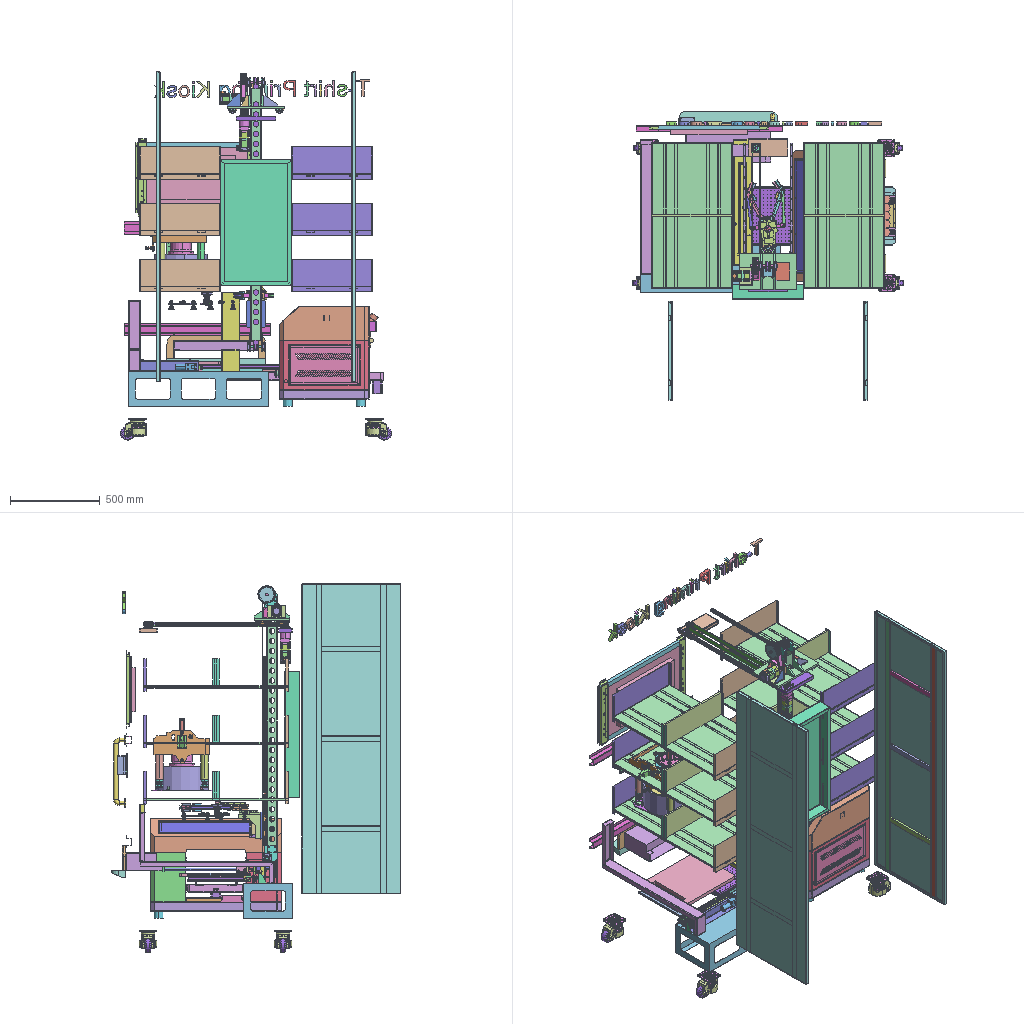Assembly | SolidWorks | 205 different items | 337 placed | box 1506 x 1606 x 2047 mm
Parts list (item | name | quantity | parent item | size | volume | features):
1 | (subassembly) | x1 | in 35 | - | 6869314 mm3 | -
2 | (subassembly) | x1 | in 1 | 730 x 556.8 x 540 mm | 4115428 mm3 | -
3 | (subassembly) | x1 | in 2 | 730 x 190.8 x 500 mm | 1142428 mm3 | -
4 | (subassembly) | x1 | in 1 | 51.5 x 40 x 94 mm | 58033 mm3 | -
5 | (subassembly) | x1 | in 1 | 1.2 x 37 x 16 mm | 407.189 mm3 | -
6 | (subassembly) | x1 | in 9 | 30.5 x 22 x 22 mm | 4805 mm3 | -
7 | (subassembly) | x1 | in 35 | - | 5211065 mm3 | -
8 | (subassembly) | x1 | in 7 | 56.4 x 106.5 x 56.4 mm | 231072 mm3 | -
9 | (subassembly) | x1 | in 7 | 35 x 25 x 30.5 mm | 7521 mm3 | -
10 | (subassembly) | x1 | in 7 | 528 x 29.8 x 318 mm | 2287252 mm3 | -
11 | (subassembly) | x1 | in 22 | 25 x 45 x 45 mm | 14314 mm3 | -
12 | (subassembly) | x1 | in 23 | 85 x 119 x 74.5 mm | 264146 mm3 | -
13 | (subassembly) | x1 | in 23 | 22 x 26 x 26 mm | 5822 mm3 | -
14 | (subassembly) | x1 | in 23 | 32 x 26 x 26 mm | 8249 mm3 | -
15 | (subassembly) | x1 | in 23 | 22 x 33 x 33 mm | 8275 mm3 | -
16 | (subassembly) | x2 | in 23 | 32 x 52 x 52 mm | 45513 mm3 | -
17 | (subassembly) | x1 | in 23 | 32 x 99 x 99 mm | 209787 mm3 | -
18 | (subassembly) | x1 | in 7 | 40 x 895 x 39.5 mm | 383504 mm3 | -
19 | (subassembly) | x1 | in 7 | 40 x 895 x 39.5 mm | 383504 mm3 | -
20 | (subassembly) | x1 | in 26 | 220 x 80 x 232.061 mm | 626887 mm3 | -
21 | (subassembly) | x1 | in 26 | 220 x 100 x 60.061 mm | 148647 mm3 | -
22 | (subassembly) | x1 | in 26 | 410 x 73.7 x 435 mm | 472209 mm3 | -
23 | (subassembly) | x1 | in 26 | - | 4751526 mm3 | -
24 | (subassembly) | x1 | in 26 | 845 x 1628 x 281.2 mm | 12737419 mm3 | -
25 | (subassembly) | x1 | in 26 | 648 x 1628 x 92.4 mm | 1922415 mm3 | -
26 | (subassembly) | x1 | - | - | - | -
27 | (subassembly) | x1 | in 26 | 397.81 x 402.788 x 334.249 mm | 8465186 mm3 | -
28 | (subassembly) | x1 | in 26 | 47 x 24.01 x 800.23 mm | 223806 mm3 | -
29 | (subassembly) | x1 | in 26 | 47 x 24.01 x 800.23 mm | 223806 mm3 | -
30 | (subassembly) | x1 | in 26 | 1502 x 997.4 x 1969 mm | 40879117 mm3 | -
31 | (subassembly) | x1 | in 32 | 42.13 x 42.13 x 71 mm | 53858 mm3 | -
32 | (subassembly) | x1 | in 26 | 350 x 121.3 x 561.8 mm | 585009 mm3 | -
33 | (subassembly) | x1 | in 23 | 57 x 57 x 106 mm | 252225 mm3 | -
34 | (subassembly) | x2 | in 20, 23 | 70 x 57 x 138 mm | 311067 mm3 | -
35 | (subassembly) | x1 | in 26 | - | 12080386 mm3 | -
36 | (subassembly) | x1 | in 2 | 730 x 429 x 540 mm | 2282239 mm3 | -
37 | - | x1 | in 22 | 48 x 13.9 x 400 mm | 34049 mm3 | features BaseBody 1
38 | - | x4 | in 23 | 30.6 x 47.8 x 30.6 mm | 8722 mm3 | features BaseBody 1
39 | - | x1 | in 32 | 56 x 70 x 515.8 mm | 426528 mm3 | features BaseBody 8
40 | - | x1 | in 21 | 18 x 60 x 18 mm | 10992 mm3 | features BaseBody 1
41 | - | x2 | in 26 | 848 x 1486 x 20 mm | 1659085 mm3 | features BaseBody 6
42 | - | x1 | in 24 | 200 x 100 x 472.4 mm | 283368 mm3 | features BaseBody 1
43 | - | x1 | in 24 | 550 x 140 x 20 mm | 564852 mm3 | features BaseBody 1
44 | - | x1 | in 24 | 94 x 132 x 55 mm | 461211 mm3 | features BaseBody 3
45 | - | x2 | in 24 | 70 x 31 x 812 mm | 103469 mm3 | features BaseBody 1
46 | - | x1 | in 27 | 300.482 x 402.788 x 300.482 mm | 4049858 mm3 | features BaseBody 27, Scale 1
47 | - | x1 | in 27 | 371.182 x 272.09 x 310.892 mm | 3352591 mm3 | features BaseBody 47, ICE 1, Scale 1
48 | - | x2 | in 22 | - | - | features BaseBody 1, RefSurface 1
49 | - | x4 | in 27 | 42.588 x 252.216 x 42.588 mm | 265706 mm3 | features BaseBody 1, Scale 1
50 | - | x1 | in 26 | 1198 x 114.943 x 20 mm | 636251 mm3 | features BaseBody 24
51 | - | x1 | in 24 | 845 x 1628 x 31.2 mm | 1603830 mm3 | features BaseBody 1
52 | - | x4 | in 23 | 85 x 100 x 6 mm | 36550 mm3 | features BaseBody 1
53 | - | x2 | in 26 | 549 x 1721 x 20 mm | 1317735 mm3 | features BaseBody 6
54 | - | x1 | in 23 | 280 x 40 x 14 mm | 34482 mm3 | features BaseBody 1
55 | - | x2 | in 23 | 260 x 25 x 4 mm | 24301 mm3 | features BaseBody 1
56 | - | x1 | in 25 | 524 x 524 x 91.2 mm | 502575 mm3 | features BaseBody 1
57 | - | x1 | in 26 | 701.5 x 477 x 103 mm | 268685 mm3 | features BaseBody 1
58 | - | x1 | in 26 | 751.5 x 394 x 68 mm | 198478 mm3 | features BaseBody 1
59 | - | x1 | in 22 | 40 x 60 x 390 mm | 67667 mm3 | features BaseBody 3
60 | - | x1 | in 21 | 50 x 50 x 2.5 mm | 2837 mm3 | features BaseBody 1
61 | - | x1 | in 23 | 40 x 60 x 6 mm | 13211 mm3 | features BaseBody 1
62 | - | x5 | in 1 | 45 x 111.906 x 127 mm | 412222 mm3 | features BaseBody 1
63 | - | x1 | in 26 | 470 x 160 x 420 mm | 277049 mm3 | features BaseBody 1
64 | - | x1 | in 23 | 20 x 75 x 20 mm | 9389 mm3 | features BaseBody 1
65 | - | x6 | in 26 | 809.4 x 448 x 181.2 mm | 1546539 mm3 | features BaseBody 8
66 | - | x1 | in 25 | 648 x 1628 x 71.2 mm | 1419840 mm3 | features BaseBody 2
67 | - | x1 | in 26 | 780 x 270 x 193 mm | 595214 mm3 | features BaseBody 1
68 | - | x1 | in 1 | 40.5 x 77 x 40.5 mm | 60164 mm3 | features BaseBody 1
69 | - | x1 | in 21 | 220 x 100 x 22.5 mm | 80575 mm3 | features BaseBody 1
70 | - | x1 | in 22 | 118 x 73 x 40 mm | 109791 mm3 | features BaseBody 2
71 | - | x2 | in 23, 26 | 320 x 200 x 12 mm | 721363 mm3 | features BaseBody 1
72 | - | x1 | in 1 | 160 x 95 x 11.5 mm | 41578 mm3 | features BaseBody 1
73 | - | x1 | in 22 | 350 x 83 x 13.5 mm | 34272 mm3 | features BaseBody 1
74 | - | x1 | in 32 | 43 x 350 x 21.5 mm | 41885 mm3 | features BaseBody 1
75 | - | x1 | in 23 | 80 x 400 x 12 mm | 339060 mm3 | features BaseBody 1
76 | - | x2 | in 23 | 120 x 135 x 12 mm | 77989 mm3 | features BaseBody 1
77 | - | x2 | in 23 | 200 x 60 x 10 mm | 88500 mm3 | features BaseBody 1
78 | - | x1 | in 23 | 80 x 60 x 100 mm | 48337 mm3 | features BaseBody 3
79 | - | x1 | in 23 | 40 x 60 x 100 mm | 31587 mm3 | features BaseBody 3
80 | - | x1 | in 24 | 80 x 40 x 550 mm | 1225633 mm3 | features BaseBody 1
81 | - | x1 | in 22 | 40 x 40 x 3 mm | 4208 mm3 | features BaseBody 1
82 | - | x1 | in 26 | 370.752 x 47.5 x 215.235 mm | 560908 mm3 | features Simplified 1
83 | - | x1 | in 1 | 35 x 89.2 x 119.2 mm | 310275 mm3 | features BaseBody 1
84 | - | x1 | in 32 | 42 x 32 x 60 mm | 48942 mm3 | features BaseBody 1
85 | - | x1 | in 20 | 220 x 80 x 28.5 mm | 68987 mm3 | features BaseBody 5
86 | - | x1 | in 23 | 72.5 x 72.5 x 100 mm | 47696 mm3 | features BaseBody 3
87 | - | x1 | in 26 | 397.4 x 702.4 x 82.4 mm | 594680 mm3 | features BaseBody 1
88 | - | x1 | in 26 | 44.42 x 804.42 x 25 mm | 82663 mm3 | features BaseBody 1
89 | - | x1 | in 22 | 365.37 x 34.87 x 15 mm | 22928 mm3 | features BaseBody 1
90 | - | x1 | in 23 | 1519 x 50.79 x 25 mm | 154464 mm3 | features BaseBody 1
91 | - | x1 | in 23 | 153.425 x 115.925 x 25 mm | 20675 mm3 | features BaseBody 1
92 | - | x1 | in 10 | 310 x 10 x 520 mm | 1611142 mm3 | features BaseBody 1
93 | - | x1 | in 23 | 182.982 x 147.508 x 15 mm | 14200 mm3 | features BaseBody 1
94 | - | x1 | in 23 | 118 x 73 x 40 mm | 109791 mm3 | features BaseBody 2
95 | - | x10 | in 23, 28, 29 | 47 x 19.61 x 65.8 mm | 33744 mm3 | features BaseBody 6
96 | - | x1 | in 23 | 15 x 15 x 1050 mm | 206865 mm3 | features BaseBody 1
97 | - | x2 | in 28, 29 | 15 x 15 x 800 mm | 156317 mm3 | features BaseBody 1
98 | - | x2 | in 23 | 8.5 x 16.5 x 9.238 mm | 659.616 mm3 | features BaseBody 1
99 | - | x1 | in 1 | 30 x 28 x 400 mm | 43012 mm3 | features BaseBody 1
100 | - | x2 | in 1 | 30 x 28 x 170 mm | 18284 mm3 | features BaseBody 1
101 | - | x1 | in 1 | 30 x 28 x 330 mm | 35652 mm3 | features BaseBody 1
102 | - | x1 | in 1 | 30 x 28 x 420 mm | 45183 mm3 | features BaseBody 1
103 | - | x4 | in 26 | 139.5 x 98 x 120 mm | 590754 mm3 | features BaseBody 7
104 | - | x2 | in 1 | 30 x 28 x 100 mm | 10719 mm3 | features BaseBody 1
105 | - | x1 | in 1 | 72 x 2 x 53 mm | 7555 mm3 | features BaseBody 1
106 | - | x4 | in 2 | 50 x 40 x 50 mm | 78540 mm3 | features BaseBody 1
107 | - | x2 | in 26 | 320 x 445 x 20 mm | 2654283 mm3 | features BaseBody 1
108 | - | x4 | in 30 | 200 x 21.2 x 1000 mm | 392351 mm3 | features BaseBody 1
109 | - | x1 | in 32 | 80 x 41.5 x 60 mm | 13821 mm3 | features BaseBody 1
110 | - | x1 | in 23 | 110 x 150 x 10 mm | 158649 mm3 | features BaseBody 1
111 | - | x1 | in 24 | 400 x 68.5 x 50 mm | 236028 mm3 | features BaseBody 1
112 | - | x2 | in 30 | 41 x 61 x 1488 mm | 193542 mm3 | features BaseBody 1
113 | - | x2 | in 30 | 92.2 x 216 x 1489 mm | 543457 mm3 | features BaseBody 1
114 | - | x2 | in 23 | 40.2 x 13.5 x 26.6 mm | 5331 mm3 | features BaseBody 1
115 | - | x1 | in 24 | 654.7 x 392.6 x 50 mm | 8081843 mm3 | features BaseBody 2
116 | - | x2 | in 34 | 57 x 57 x 20 mm | 26453 mm3 | features BaseBody 1
117 | - | x2 | in 22 | 22 x 36 x 36 mm | 13261 mm3 | features BaseBody 1
118 | - | x1 | in 33 | 57 x 57 x 61 mm | 178844 mm3 | features BaseBody 1
119 | - | x1 | in 33 | 57 x 57 x 13 mm | 37451 mm3 | features BaseBody 1
120 | - | x2 | in 34 | 57 x 57 x 41 mm | 117011 mm3 | features BaseBody 1
121 | - | x2 | in 34 | 57 x 13 x 57 mm | 37051 mm3 | features BaseBody 1
122 | - | x2 | in 34 | 57 x 31 x 57 mm | 87629 mm3 | features BaseBody 1
123 | - | x2 | in 34 | 57 x 57 x 33 mm | 37132 mm3 | features BaseBody 1
124 | - | x1 | in 20 | 57 x 57 x 110 mm | 214334 mm3 | features BaseBody 1
125 | - | x1 | in 23 | 60 x 60 x 1400 mm | 753847 mm3 | features BaseBody 1
126 | - | x2 | in 2 | 80 x 25 x 102 mm | 111075 mm3 | features BaseBody 1
127 | - | x1 | in 12 | 82 x 82 x 5 mm | 7163 mm3 | features BaseBody 1
128 | - | x1 | in 22 | 35 x 32 x 6 mm | 5233 mm3 | features BaseBody 1
129 | - | x1 | in 1 | 49.7 x 29.1 x 21.7 mm | 6028 mm3 | features BaseBody 1
130 | - | x1 | in 36 | 730 x 58.5 x 500 mm | 825943 mm3 | features BaseBody 1
131 | - | x1 | in 36 | 199 x 275 x 500 mm | 589310 mm3 | features BaseBody 1
132 | - | x1 | in 36 | 199 x 275 x 500 mm | 597228 mm3 | features BaseBody 1
133 | - | x1 | in 36 | 600 x 104 x 197 mm | 256427 mm3 | features BaseBody 3
134 | - | x2 | in 36 | 70 x 1.5 x 100 mm | 6665 mm3 | features BaseBody 1
135 | - | x1 | in 3 | 730 x 190 x 500 mm | 771192 mm3 | features BaseBody 1
136 | - | x2 | in 2 | 388 x 215 x 1 mm | 77225 mm3 | features BaseBody 1
137 | - | x1 | in 4 | 18 x 40 x 35 mm | 1986 mm3 | features BaseBody 1
138 | - | x1 | in 7 | 325 x 42 x 910 mm | 886307 mm3 | features BaseBody 1
139 | - | x1 | in 22 | 8 x 8 x 65 mm | 3128 mm3 | features BaseBody 1
140 | - | x1 | in 7 | 134 x 7.2 x 760 mm | 132478 mm3 | features BaseBody 1
141 | - | x2 | in 7 | 49.5 x 10.7 x 760 mm | 52509 mm3 | features BaseBody 1
142 | - | x2 | in 7 | 210 x 11 x 65 mm | 28784 mm3 | features BaseBody 1
143 | - | x1 | in 10 | 520 x 17.8 x 225 mm | 330533 mm3 | features BaseBody 1
144 | - | x1 | in 10 | 528 x 9 x 318 mm | 345577 mm3 | features BaseBody 1
145 | - | x1 | in 7 | 520 x 25 x 310 mm | 696143 mm3 | features BaseBody 1
146 | - | x1 | in 3 | 628 x 2 x 198 mm | 248418 mm3 | features BaseBody 1
147 | - | x1 | in 3 | 628 x 2 x 98 mm | 122818 mm3 | features BaseBody 1
148 | - | x1 | in 5 | 37 x 1.2 x 16 mm | 407.189 mm3 | features BaseBody 1
149 | - | x2 | in 7 | 16 x 18.5 x 30 mm | 1165 mm3 | features BaseBody 1
150 | - | x2 | in 11 | 1 x 21.856 x 23 mm | 128.626 mm3 | features BaseBody 1
151 | - | x2 | in 7 | 16 x 25.5 x 60 mm | 4352 mm3 | features BaseBody 1
152 | - | x2 | in 7 | 60 x 2 x 24 mm | 2796 mm3 | features BaseBody 1
153 | - | x1 | in 9 | 23.3 x 35 x 25 mm | 2716 mm3 | features BaseBody 1
154 | - | x1 | in 6 | 8 x 29 x 10 mm | 861.581 mm3 | features BaseBody 1
155 | - | x1 | in 1 | 19 x 43.7 x 19 mm | 9001 mm3 | features BaseBody 2
156 | - | x1 | in 30 | 1502 x 997.4 x 1969 mm | 37461315 mm3 | features BaseBody 37
157 | - | x16 | in 30 | 80 x 80 x 6 mm | 23400 mm3 | features BaseBody 1
158 | - | x1 | in 4 | 24 x 85 x 50.5 mm | 56047 mm3 | features BaseBody 1
159 | - | x1 | in 1 | 19 x 53.2 x 19 mm | 10652 mm3 | features BaseBody 2
160 | - | x4 | in 1, 7 | 44 x 20.7 x 11 mm | 3616 mm3 | features BaseBody 1
161 | - | x1 | in 22 | 28 x 26.1 x 88 mm | 25740 mm3 | features BaseBody 1
162 | - | x1 | in 12 | 8 x 4 x 4 mm | 90.792 mm3 | features BaseBody 1
163 | - | x12 | in 12 | 13 x 5.5 x 5.5 mm | 133.192 mm3 | features BaseBody 1
164 | - | x9 | in 12 | 25 x 8.5 x 8.5 mm | 634.476 mm3 | features BaseBody 1
165 | - | x2 | in 6 | 5 x 15 x 15 mm | 413.271 mm3 | features BaseBody 16
166 | - | x1 | in 12 | 85 x 119 x 22 mm | 77366 mm3 | features BaseBody 1
167 | - | x1 | in 12 | 6 x 78.9 x 78.9 mm | 13059 mm3 | features BaseBody 1
168 | - | x1 | in 12 | 22.5 x 70 x 70 mm | 47799 mm3 | features BaseBody 2
169 | - | x1 | in 12 | 39 x 38.986 x 10 mm | 8129 mm3 | features BaseBody 1
170 | - | x1 | in 12 | 22 x 60 x 60 mm | 35107 mm3 | features BaseBody 1
171 | - | x1 | in 12 | 48.8 x 24 x 24 mm | 9180 mm3 | features BaseBody 1
172 | - | x1 | in 22 | 32 x 17.5 x 400 mm | 119366 mm3 | features BaseBody 1
173 | - | x1 | in 12 | 26 x 60 x 60 mm | 48842 mm3 | features BaseBody 1
174 | - | x1 | in 13 | 22 x 26 x 26 mm | 5766 mm3 | features BaseBody 1
175 | - | x1 | in 14 | 32 x 26 x 26 mm | 8249 mm3 | features BaseBody 1
176 | - | x1 | in 15 | 22 x 33 x 33 mm | 8275 mm3 | features BaseBody 1
177 | - | x2 | in 16 | 32 x 52 x 52 mm | 45513 mm3 | features BaseBody 1
178 | - | x1 | in 17 | 32 x 99 x 99 mm | 209787 mm3 | features BaseBody 1
179 | - | x1 | in 33 | 57 x 57 x 32 mm | 35610 mm3 | features BaseBody 1
180 | - | x2 | in 24 | 65 x 432 x 26.6 mm | 36858 mm3 | features BaseBody 1
181 | - | x1 | in 6 | 9 x 10 x 9 mm | 179.425 mm3 | features BaseBody 1
182 | - | x2 | in 12 | 9 x 37 x 37 mm | 5051 mm3 | features BaseBody 1
183 | - | x2 | in 11 | 7 x 22 x 22 mm | 2095 mm3 | features BaseBody 1
184 | - | x2 | in 34 | 33.5 x 13 x 32 mm | 5786 mm3 | features BaseBody 1
185 | - | x1 | in 6 | 15 x 22 x 22 mm | 2686 mm3 | features BaseBody 1
186 | - | x2 | in 8 | 23 x 22 x 22 mm | 5516 mm3 | features BaseBody 1
187 | - | x2 | in 18, 19 | 30 x 895 x 28.5 mm | 320903 mm3 | features BaseBody 1
188 | - | x4 | in 18, 19 | 40 x 39 x 27.6 mm | 31300 mm3 | features BaseBody 1
189 | - | x2 | in 13 | 3 x 4 x 4 mm | 27.73 mm3 | features BaseBody 1
190 | - | x1 | in 8 | 56.4 x 106.5 x 56.4 mm | 220040 mm3 | features BaseBody 1
191 | - | x1 | in 23 | 15 x 15 x 150 mm | 26507 mm3 | features BaseBody 1
192 | - | x1 | in 23 | 15 x 15 x 100 mm | 17671 mm3 | features BaseBody 1
193 | - | x1 | in 7 | 695.6 x 10 x 20.6 mm | 16931 mm3 | features BaseBody 1
194 | - | x1 | in 22 | 57.5 x 20.5 x 45 mm | 2654 mm3 | features BaseBody 1
195 | - | x1 | in 31 | 69 x 5 x 5 mm | 1331 mm3 | features BaseBody 1
196 | - | x1 | in 31 | 42.13 x 42.13 x 30 mm | 33535 mm3 | features BaseBody 1
197 | - | x4 | in 31 | 41.388 x 5.6 x 5.6 mm | 251.599 mm3 | features BaseBody 1
198 | - | x1 | in 31 | 42 x 42 x 12 mm | 8860 mm3 | features BaseBody 1
199 | - | x1 | in 31 | 42 x 42 x 11 mm | 9125 mm3 | features BaseBody 1
200 | - | x5 | in 33 | 6 x 3 x 6 mm | 63.932 mm3 | features BaseBody 1
201 | - | x2 | in 20, 21 | 32.122 x 48 x 48 mm | 32488 mm3 | features BaseBody 1
202 | - | x2 | in 6 | 3.5 x 10 x 10 mm | 125.675 mm3 | features BaseBody 1
203 | - | x6 | in 21, 23 | 63 x 63 x 17 mm | 21756 mm3 | features BaseBody 14
204 | - | x1 | in 23 | 34.5 x 33.2 x 19.63 mm | 7219 mm3 | features BaseBody 1
205 | - | x1 | in 11 | 25 x 45 x 45 mm | 9867 mm3 | features BaseBody 1
Mates (type | each side: item.copy, entity, surface, feature):
In subassembly 26
Coincident | 127.1 face plane 输入1 | 82.1 face
Coincident | 65.1 face plane 输入1 | 47.1 face plane 输入68
Parallel | 65.1 face plane 输入8 | 47.1 face plane 输入68
In subassembly 27
Concentric | 47.2 face cylinder 输入10 | 46.1 face cylinder 输入16
Concentric | 47.2 face cylinder 输入1 | 49.1 face cylinder 输入1
Coincident | 47.2 face plane 输入68 | 49.1 face plane 输入1
Concentric | 47.2 face cylinder 输入68 | 49.2 face cylinder 输入1
Coincident | 47.2 face plane 输入68 | 49.2 face plane 输入1
Concentric | 47.2 face cylinder 输入4 | 49.3 face cylinder 输入1
Coincident | 47.2 face plane 输入68 | 49.3 face plane 输入1
Concentric | 47.2 face cylinder 输入2 | 49.4 face cylinder 输入1
Coincident | 47.2 face plane 输入68 | 49.4 face plane 输入1
Coincident | 47.2 face plane 输入66 | 46.1 face plane 输入15